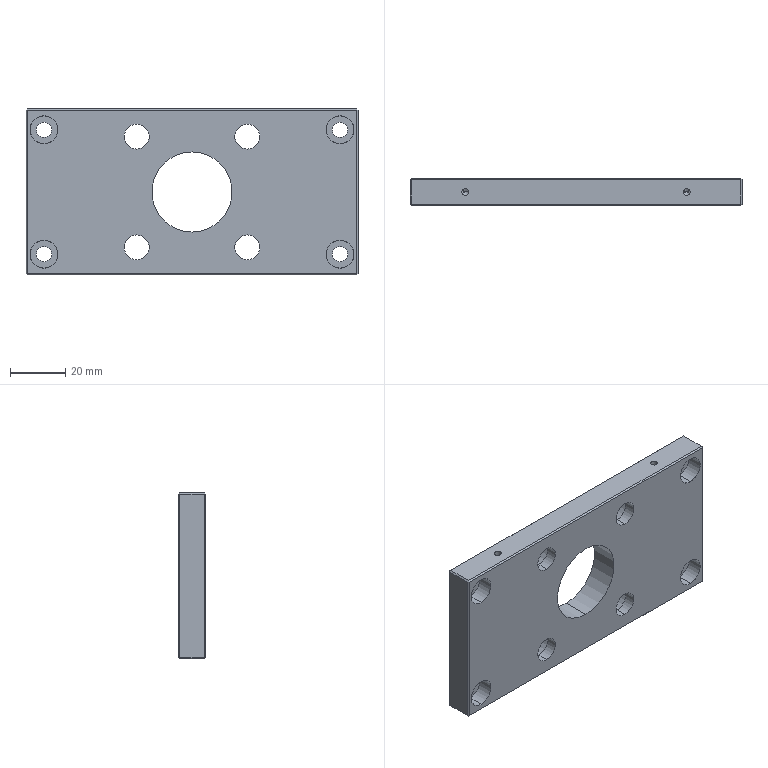Part | SolidWorks | features HoleWzd 3, ICE 2, Chamfer 1, Extrusion 1 | 1 solid | 92 faces | box 120 x 10 x 60 mm | volume 57722 mm3 | cylinder 38 | plane 34 | cone 20 | commonest cylinder face diameters 5.5 x8 9 x8 10 x8 15 x8 2.5 x4 29 x2